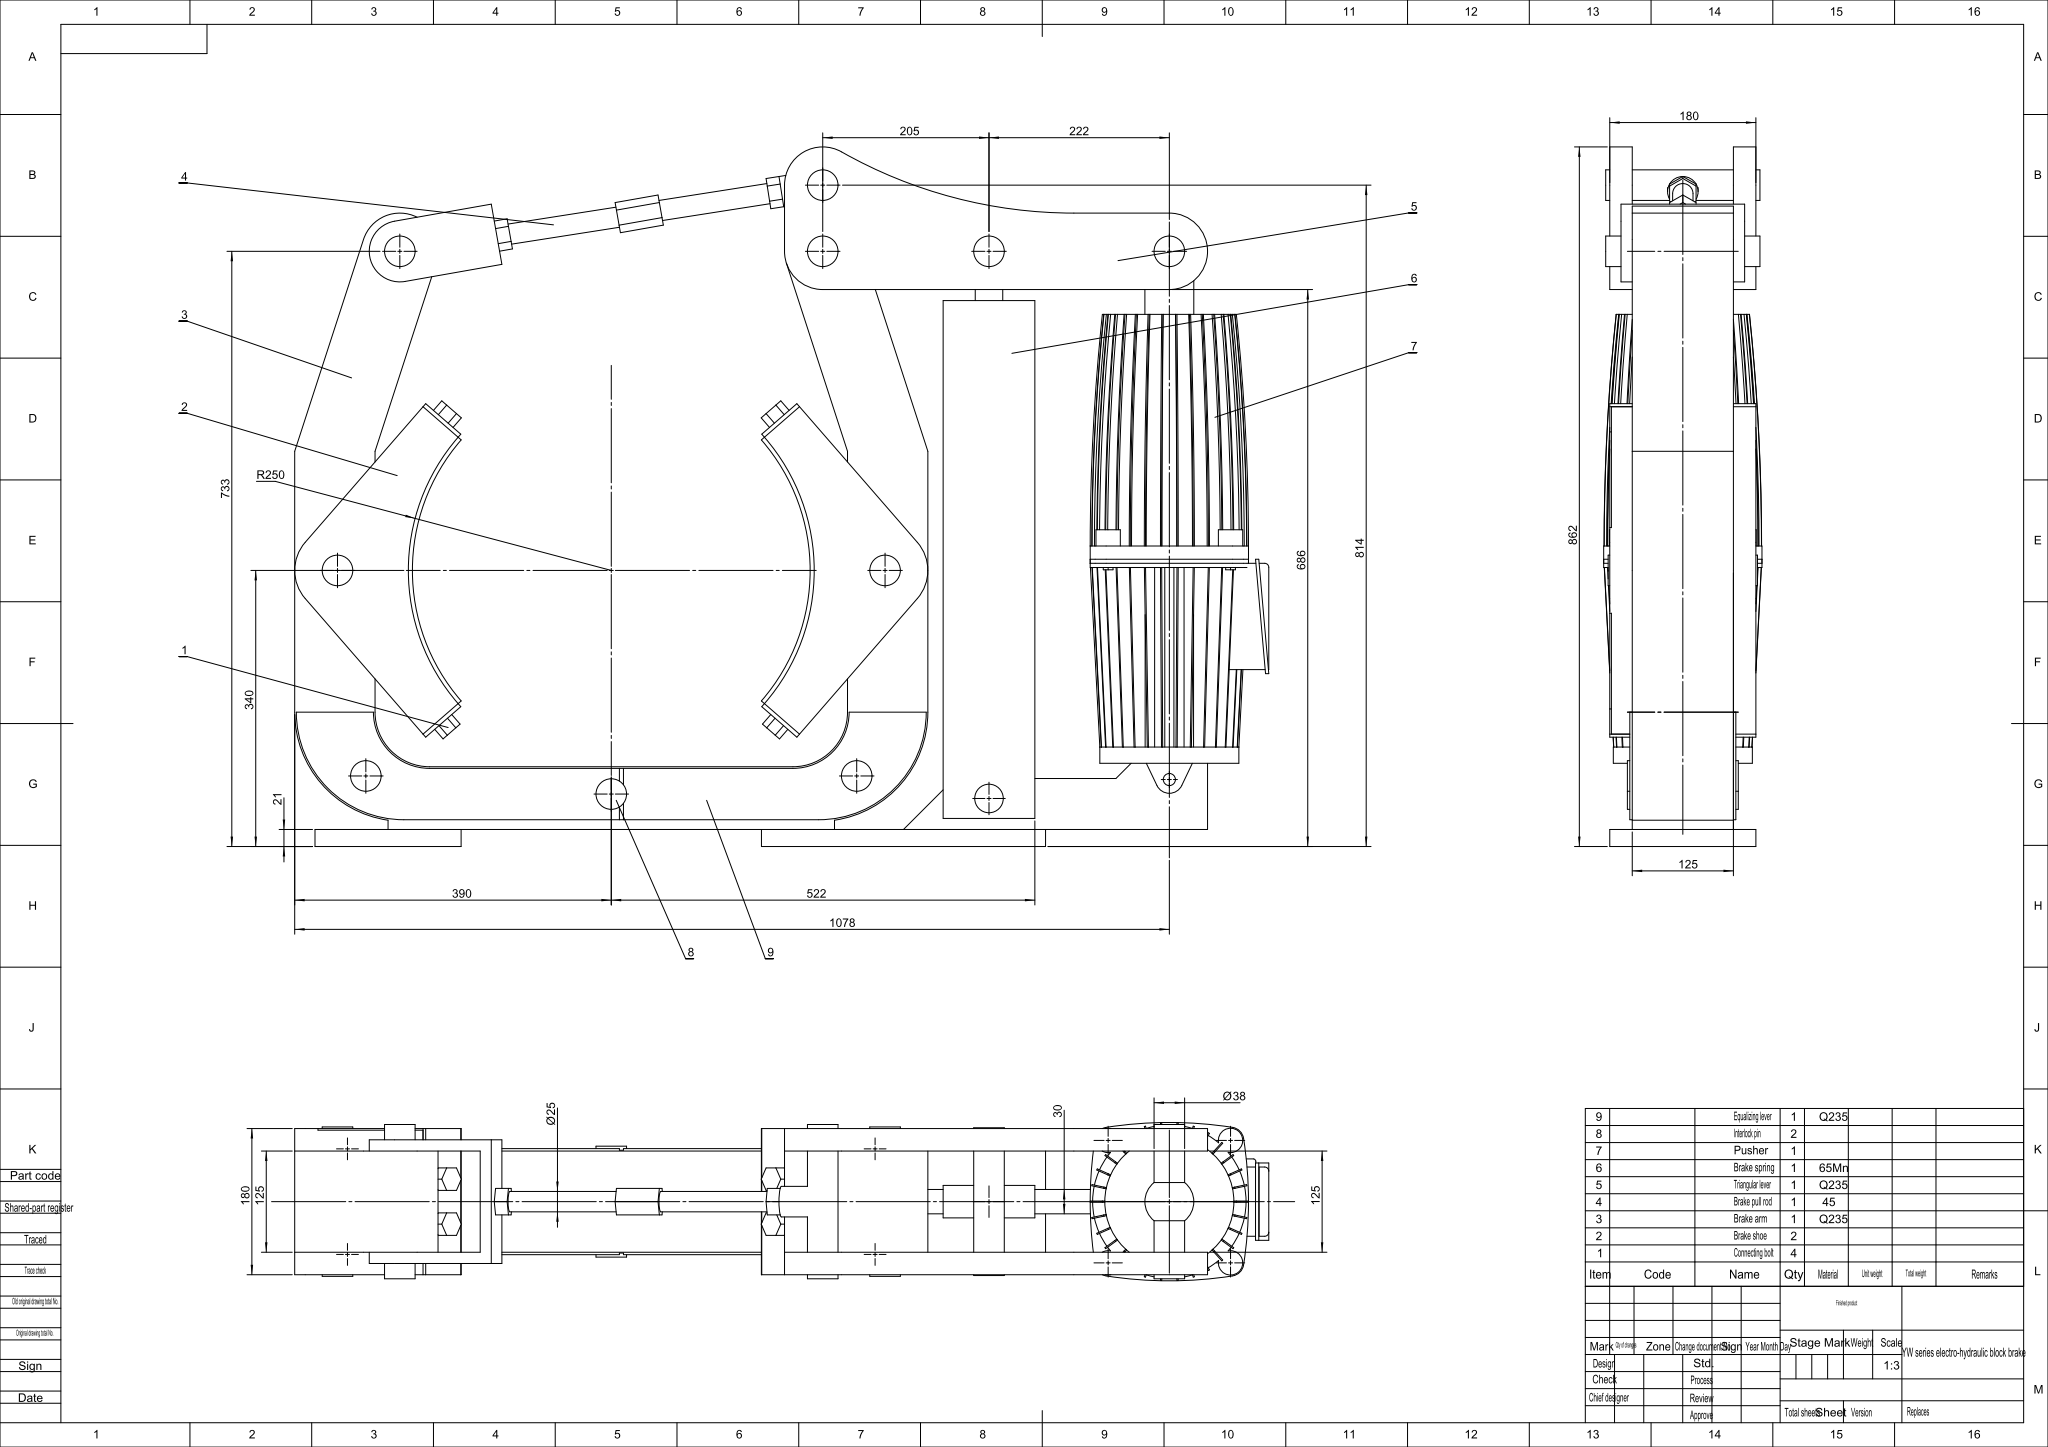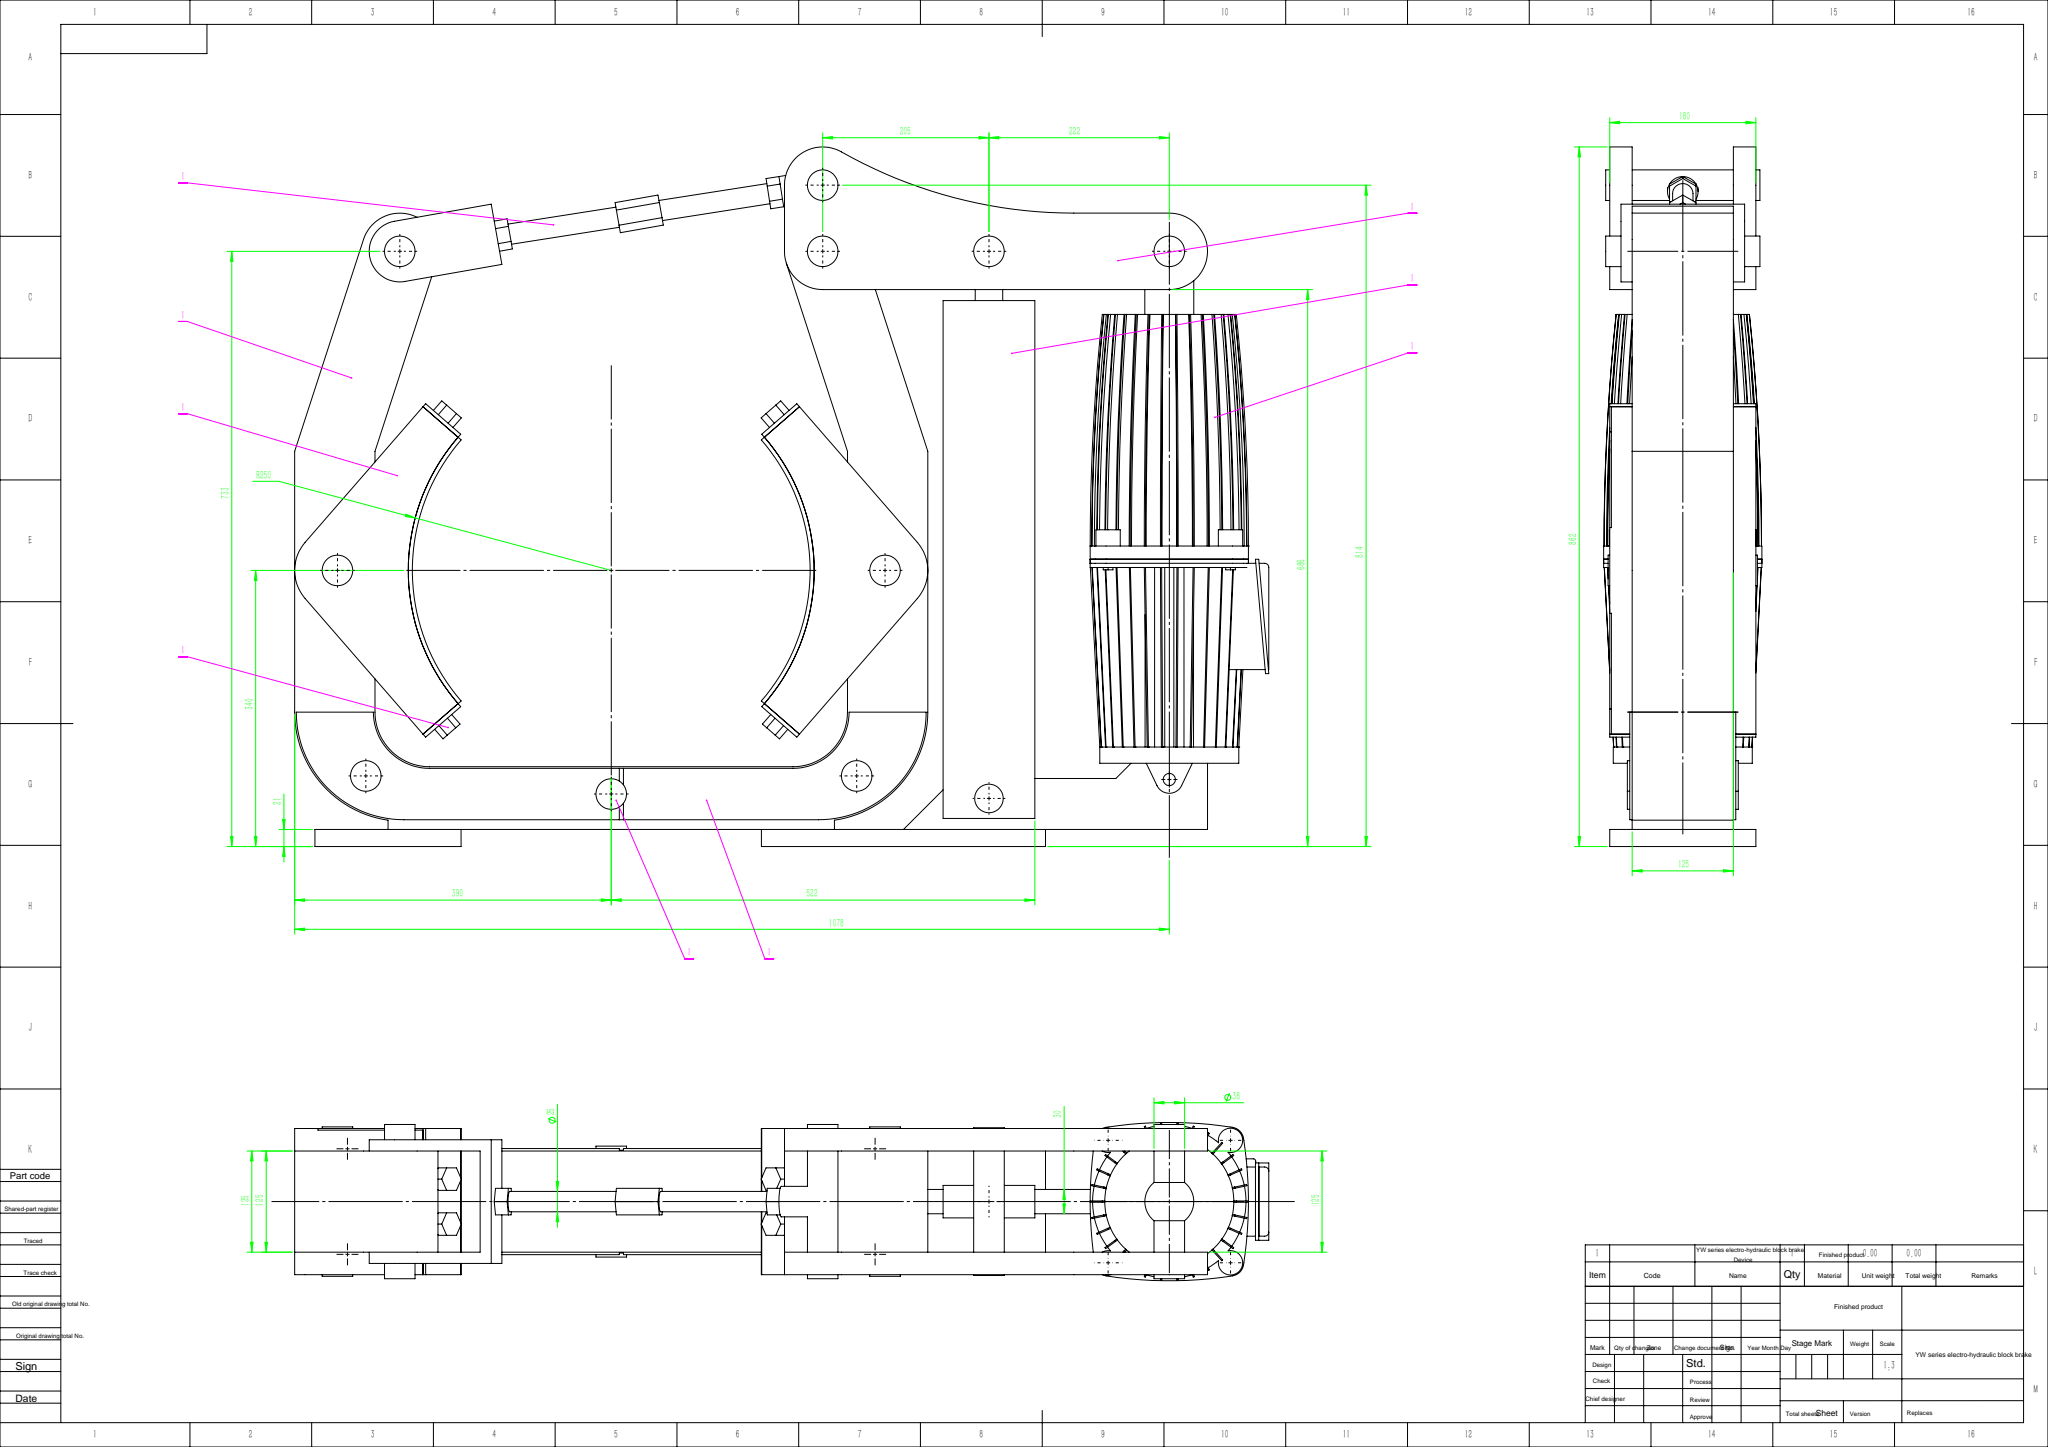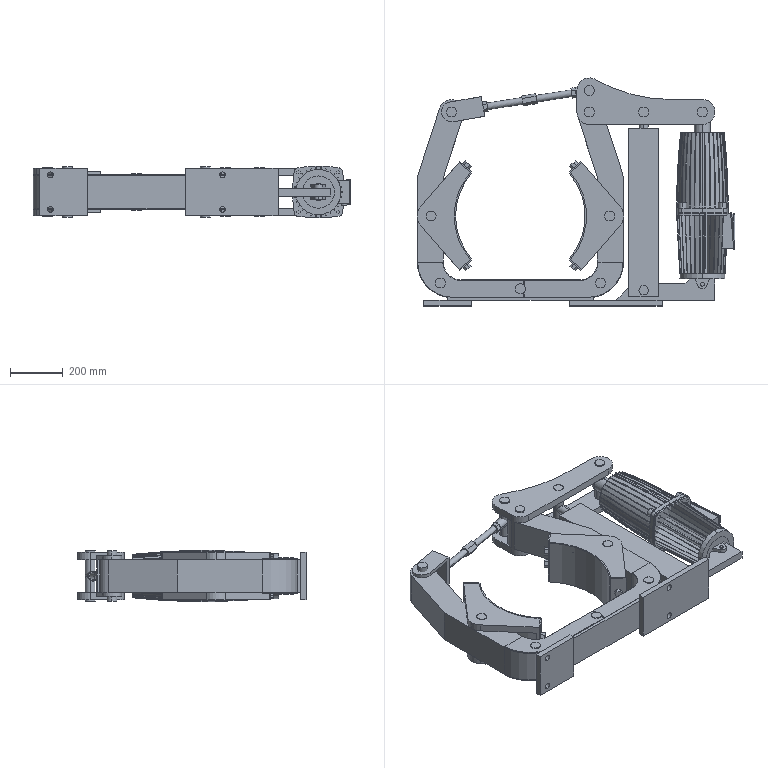Part | SolidWorks | features Boss 43, Fillet 5, MirrorPattern 5, Cut 4, CombineBodies 3, CirPattern 2, Revolution 2, Extrusion 1, MirrorSolid 1 | 80 solids | 876 faces | box 1200 x 861.523 x 195 mm | volume 52258785 mm3 | plane 637 | cylinder 233 | torus 4 | sphere 2 | commonest cylinder face diameters 37.654 x50 5440 x30 5446 x30 1009 x15 32.499 x12 500 x9